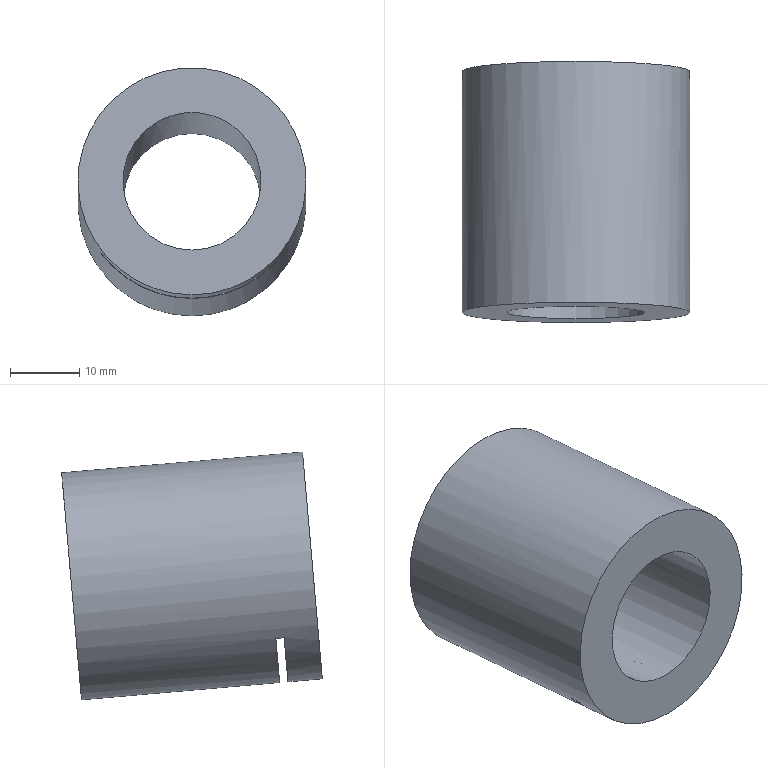Part | NX | features solid 2 | 1 solid | 7 faces | box 33 x 37.743 x 35.925 mm | volume 18800 mm3 | plane 5 | cylinder 2 | commonest cylinder face diameters 20 x1 33 x1
STEP:
#1=CARTESIAN_POINT('',(-322.976,-78.748,-18.957));
#2=VERTEX_POINT('',#1);
#3=CARTESIAN_POINT('',(-322.976,-80.186,-35.394));
#4=DIRECTION('',(0.,0.9962,-0.08716));
#5=DIRECTION('',(0.,0.08716,0.9962));
#6=AXIS2_PLACEMENT_3D('',#3,#4,#5);
#7=CIRCLE('',#6,16.5);
#8=EDGE_CURVE('',#2,#2,#7,.F.);
#9=ORIENTED_EDGE('',*,*,#8,.T.);
#10=EDGE_LOOP('',(#9));
#11=FACE_BOUND('',#10,.T.);
#12=CARTESIAN_POINT('',(-322.976,-116.491,-48.781));
#13=VERTEX_POINT('',#12);
#14=CARTESIAN_POINT('',(-322.976,-115.053,-32.344));
#15=DIRECTION('',(0.,-0.9962,0.08716));
#16=DIRECTION('',(0.,-0.08716,-0.9962));
#17=AXIS2_PLACEMENT_3D('',#14,#15,#16);
#18=CIRCLE('',#17,16.5);
#19=EDGE_CURVE('',#13,#13,#18,.T.);
#20=ORIENTED_EDGE('',*,*,#19,.F.);
#21=EDGE_LOOP('',(#20));
#22=FACE_BOUND('',#21,.T.);
#23=CARTESIAN_POINT('',(-309.928,-110.952,-42.841));
#24=VERTEX_POINT('',#23);
#25=CARTESIAN_POINT('',(-309.928,-109.757,-42.946));
#26=VERTEX_POINT('',#25);
#27=CARTESIAN_POINT('',(-309.928,-74.093,-46.066));
#28=DIRECTION('',(0.,-0.9962,0.08716));
#29=VECTOR('',#28,1000.);
#30=LINE('',#27,#29);
#31=EDGE_CURVE('',#24,#26,#30,.F.);
#32=ORIENTED_EDGE('',*,*,#31,.T.);
#33=CARTESIAN_POINT('',(-336.024,-109.757,-42.946));
#34=VERTEX_POINT('',#33);
#35=CARTESIAN_POINT('',(-322.976,-108.877,-32.884));
#36=DIRECTION('',(0.,-0.9962,0.08716));
#37=DIRECTION('',(0.,-0.08716,-0.9962));
#38=AXIS2_PLACEMENT_3D('',#35,#36,#37);
#39=CIRCLE('',#38,16.5);
#40=EDGE_CURVE('',#26,#34,#39,.F.);
#41=ORIENTED_EDGE('',*,*,#40,.T.);
#42=CARTESIAN_POINT('',(-336.024,-110.952,-42.841));
#43=VERTEX_POINT('',#42);
#44=CARTESIAN_POINT('',(-336.024,-74.093,-46.066));
#45=DIRECTION('',(0.,-0.9962,0.08716));
#46=VECTOR('',#45,1000.);
#47=LINE('',#44,#46);
#48=EDGE_CURVE('',#34,#43,#47,.T.);
#49=ORIENTED_EDGE('',*,*,#48,.T.);
#50=CARTESIAN_POINT('',(-322.976,-110.072,-32.78));
#51=DIRECTION('',(0.,-0.9962,0.08716));
#52=DIRECTION('',(0.,-0.08716,-0.9962));
#53=AXIS2_PLACEMENT_3D('',#50,#51,#52);
#54=CIRCLE('',#53,16.5);
#55=EDGE_CURVE('',#24,#43,#54,.F.);
#56=ORIENTED_EDGE('',*,*,#55,.F.);
#57=EDGE_LOOP('',(#32,#41,#49,#56));
#58=FACE_BOUND('',#57,.T.);
#59=CARTESIAN_POINT('',(-322.976,-81.382,-35.29));
#60=DIRECTION('',(0.,-0.9962,0.08716));
#61=DIRECTION('',(0.,-0.08716,-0.9962));
#62=AXIS2_PLACEMENT_3D('',#59,#60,#61);
#63=CYLINDRICAL_SURFACE('',#62,16.5);
#64=ADVANCED_FACE('',(#11,#22,#58),#63,.T.);
#65=ORIENTED_EDGE('',*,*,#19,.T.);
#66=EDGE_LOOP('',(#65));
#67=FACE_BOUND('',#66,.T.);
#68=CARTESIAN_POINT('',(-322.976,-115.925,-42.306));
#69=VERTEX_POINT('',#68);
#70=CARTESIAN_POINT('',(-322.976,-115.053,-32.344));
#71=DIRECTION('',(0.,-0.9962,0.08716));
#72=DIRECTION('',(0.,-0.08716,-0.9962));
#73=AXIS2_PLACEMENT_3D('',#70,#71,#72);
#74=CIRCLE('',#73,10.);
#75=EDGE_CURVE('',#69,#69,#74,.T.);
#76=ORIENTED_EDGE('',*,*,#75,.F.);
#77=EDGE_LOOP('',(#76));
#78=FACE_BOUND('',#77,.T.);
#79=CARTESIAN_POINT('',(-322.976,-115.053,-32.344));
#80=DIRECTION('',(0.,-0.9962,0.08716));
#81=DIRECTION('',(-1.,0.,0.));
#82=AXIS2_PLACEMENT_3D('',#79,#80,#81);
#83=PLANE('',#82);
#84=ADVANCED_FACE('',(#67,#78),#83,.T.);
#85=ORIENTED_EDGE('',*,*,#75,.T.);
#86=EDGE_LOOP('',(#85));
#87=FACE_BOUND('',#86,.T.);
#88=CARTESIAN_POINT('',(-322.976,-79.315,-25.432));
#89=VERTEX_POINT('',#88);
#90=CARTESIAN_POINT('',(-322.976,-80.186,-35.394));
#91=DIRECTION('',(0.,0.9962,-0.08716));
#92=DIRECTION('',(0.,0.08716,0.9962));
#93=AXIS2_PLACEMENT_3D('',#90,#91,#92);
#94=CIRCLE('',#93,10.);
#95=EDGE_CURVE('',#89,#89,#94,.F.);
#96=ORIENTED_EDGE('',*,*,#95,.F.);
#97=EDGE_LOOP('',(#96));
#98=FACE_BOUND('',#97,.T.);
#99=CARTESIAN_POINT('',(-322.976,-67.435,-36.51));
#100=DIRECTION('',(0.,-0.9962,0.08716));
#101=DIRECTION('',(0.,-0.08716,-0.9962));
#102=AXIS2_PLACEMENT_3D('',#99,#100,#101);
#103=CYLINDRICAL_SURFACE('',#102,10.);
#104=ADVANCED_FACE('',(#87,#98),#103,.F.);
#105=ORIENTED_EDGE('',*,*,#8,.F.);
#106=EDGE_LOOP('',(#105));
#107=FACE_BOUND('',#106,.T.);
#108=ORIENTED_EDGE('',*,*,#95,.T.);
#109=EDGE_LOOP('',(#108));
#110=FACE_BOUND('',#109,.T.);
#111=CARTESIAN_POINT('',(-322.976,-80.186,-35.394));
#112=DIRECTION('',(0.,0.9962,-0.08716));
#113=DIRECTION('',(-1.,0.,0.));
#114=AXIS2_PLACEMENT_3D('',#111,#112,#113);
#115=PLANE('',#114);
#116=ADVANCED_FACE('',(#107,#110),#115,.T.);
#117=CARTESIAN_POINT('',(-336.1,-109.757,-42.946));
#118=DIRECTION('',(-1.,0.,0.));
#119=VECTOR('',#118,1000.);
#120=LINE('',#117,#119);
#121=EDGE_CURVE('',#34,#26,#120,.F.);
#122=ORIENTED_EDGE('',*,*,#121,.F.);
#123=ORIENTED_EDGE('',*,*,#40,.F.);
#124=EDGE_LOOP('',(#122,#123));
#125=FACE_BOUND('',#124,.T.);
#126=CARTESIAN_POINT('',(-336.1,-114.115,-92.756));
#127=DIRECTION('',(0.,-0.9962,0.08716));
#128=DIRECTION('',(0.,-0.08716,-0.9962));
#129=AXIS2_PLACEMENT_3D('',#126,#127,#128);
#130=PLANE('',#129);
#131=ADVANCED_FACE('',(#125),#130,.T.);
#132=ORIENTED_EDGE('',*,*,#55,.T.);
#133=CARTESIAN_POINT('',(-336.1,-110.952,-42.841));
#134=DIRECTION('',(-1.,0.,0.));
#135=VECTOR('',#134,1000.);
#136=LINE('',#133,#135);
#137=EDGE_CURVE('',#43,#24,#136,.F.);
#138=ORIENTED_EDGE('',*,*,#137,.T.);
#139=EDGE_LOOP('',(#132,#138));
#140=FACE_BOUND('',#139,.T.);
#141=CARTESIAN_POINT('',(-336.1,-115.31,-92.651));
#142=DIRECTION('',(0.,-0.9962,0.08716));
#143=DIRECTION('',(0.,-0.08716,-0.9962));
#144=AXIS2_PLACEMENT_3D('',#141,#142,#143);
#145=PLANE('',#144);
#146=ADVANCED_FACE('',(#140),#145,.F.);
#147=ORIENTED_EDGE('',*,*,#121,.T.);
#148=ORIENTED_EDGE('',*,*,#31,.F.);
#149=ORIENTED_EDGE('',*,*,#137,.F.);
#150=ORIENTED_EDGE('',*,*,#48,.F.);
#151=EDGE_LOOP('',(#147,#148,#149,#150));
#152=FACE_BOUND('',#151,.T.);
#153=CARTESIAN_POINT('',(-336.1,-110.952,-42.841));
#154=DIRECTION('',(0.,0.08716,0.9962));
#155=DIRECTION('',(0.,0.9962,-0.08716));
#156=AXIS2_PLACEMENT_3D('',#153,#154,#155);
#157=PLANE('',#156);
#158=ADVANCED_FACE('',(#152),#157,.F.);
#159=CLOSED_SHELL('',(#64,#84,#104,#116,#131,#146,#158));
#160=MANIFOLD_SOLID_BREP('',#159);
#161=(LENGTH_UNIT()NAMED_UNIT(*)SI_UNIT(.MILLI.,.METRE.));
#162=UNCERTAINTY_MEASURE_WITH_UNIT(LENGTH_MEASURE(0.00001),#161,'','');
#163=(NAMED_UNIT(*)PLANE_ANGLE_UNIT()SI_UNIT($,.RADIAN.));
#164=(NAMED_UNIT(*)SI_UNIT($,.STERADIAN.)SOLID_ANGLE_UNIT());
#165=(GEOMETRIC_REPRESENTATION_CONTEXT(3)GLOBAL_UNCERTAINTY_ASSIGNED_CONTEXT((#162))GLOBAL_UNIT_ASSIGNED_CONTEXT((#161,#163,#164))REPRESENTATION_CONTEXT('',''));
#166=ADVANCED_BREP_SHAPE_REPRESENTATION('',(#160),#165);